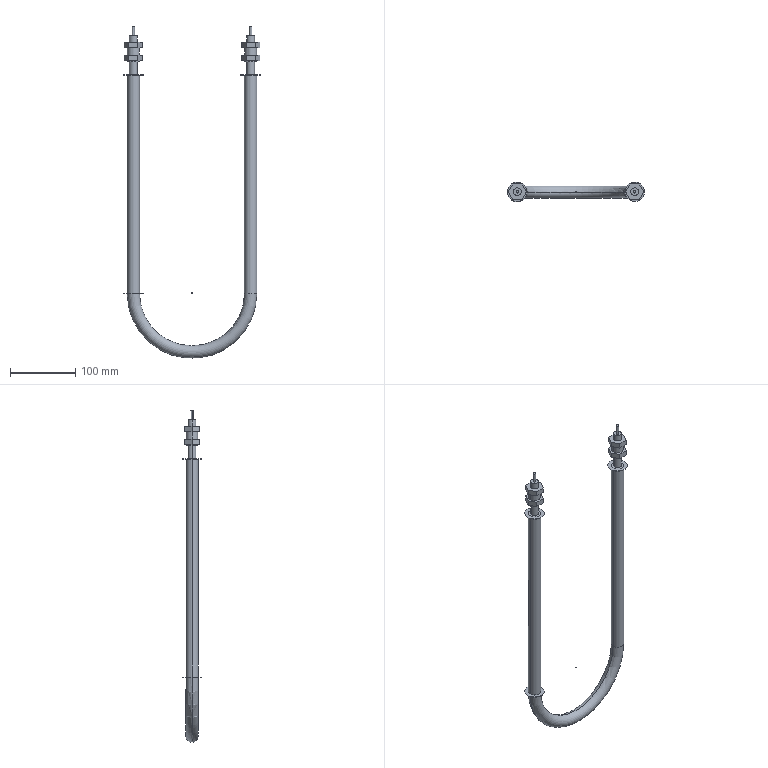Part | STEP file | Produce dryer line heating fan-HEATER-U | 2 solids | 80 faces | box 210 x 30 x 509.5 mm | volume 300889 mm3 | plane 46 | cylinder 32 | torus 2 | commonest cylinder face diameters 12 x8 18 x8 30 x6 4 x4 19 x4 1 x2